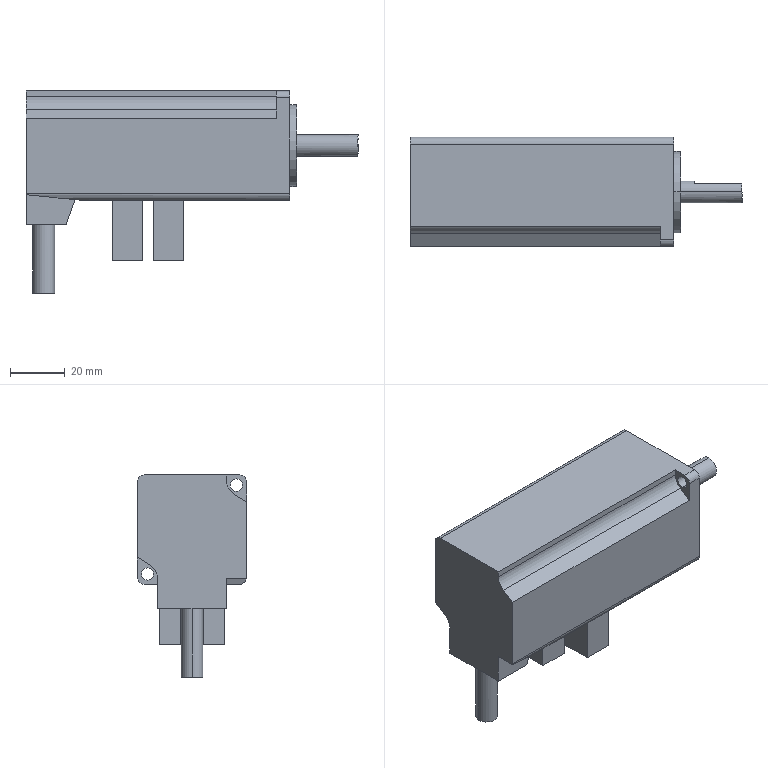Part | SolidWorks | features BaseBody 1 | 1 solid | 48 faces | box 121.5 x 40 x 74 mm | volume 159388 mm3 | plane 32 | cylinder 16 | commonest cylinder face diameters 4.5 x4 5 x4 8 x4 11.2 x2 30 x2